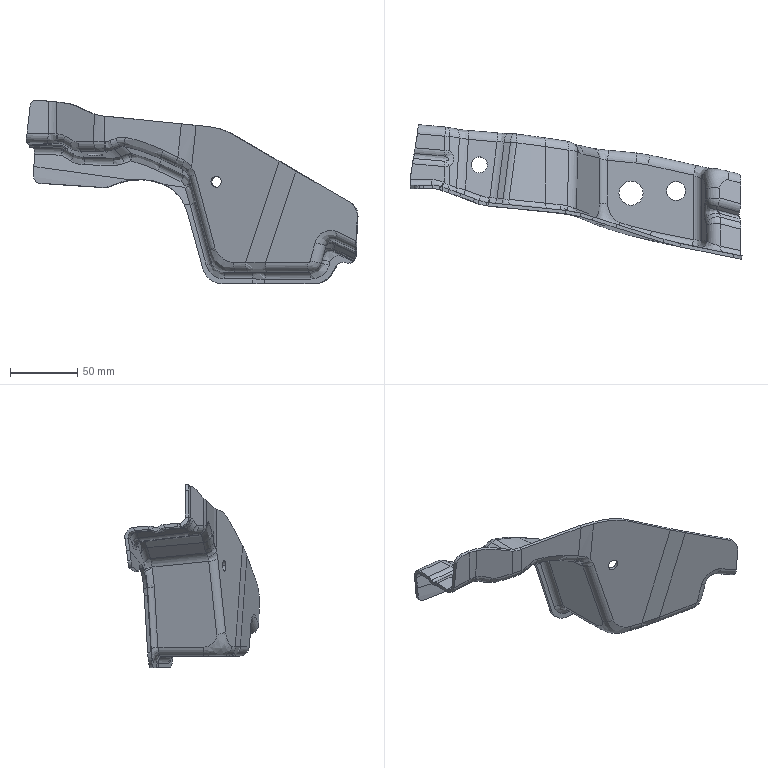Part | 1 solid | 277 faces | box 247.022 x 100.035 x 136.695 mm | volume 80961 mm3 | spline 143 | cylinder 96 | plane 21 | sphere 12 | other 5 | commonest cylinder face diameters 10 x21 15 x21 14 x14 9 x12 18 x4 12 x2